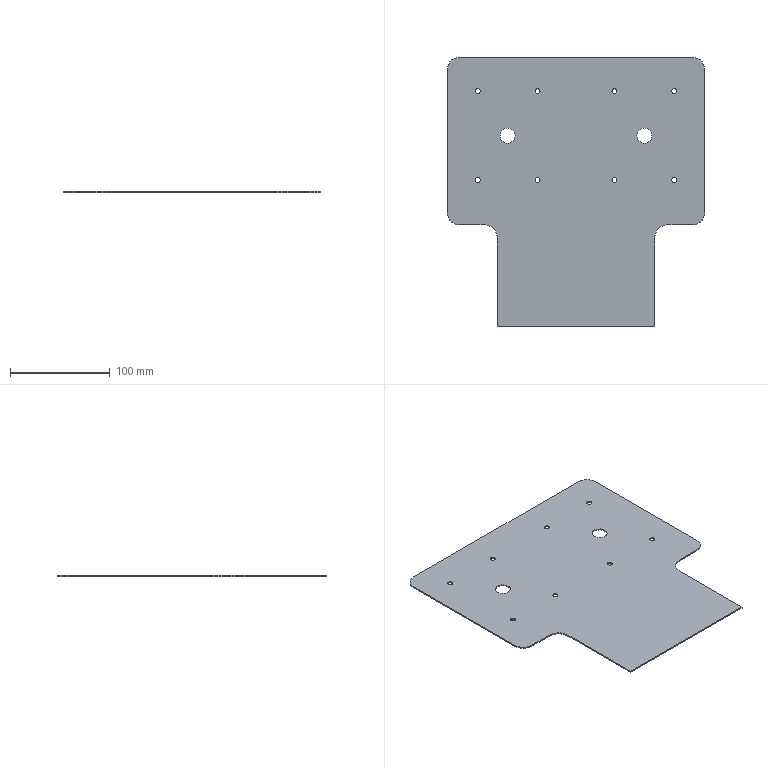Part | SolidWorks | features HoleWzd 2, FlatPattern 1, SMBaseFlange 1, SheetMetal 1 | 1 solid | 36 faces | box 257.6 x 269.6 x 1.2 mm | volume 70428 mm3 | cylinder 26 | plane 10 | commonest cylinder face diameters 5 x16 15 x4 24 x4 26.4 x2
STEP:
#1=CARTESIAN_POINT('',(-33.848,32.78,1.2));
#2=VERTEX_POINT('',#1);
#3=CARTESIAN_POINT('',(-48.848,32.78,1.2));
#4=VERTEX_POINT('',#3);
#5=CARTESIAN_POINT('',(-41.348,32.78,1.2));
#6=DIRECTION('',(0.,0.,-1.));
#7=DIRECTION('',(-1.,0.,0.));
#8=AXIS2_PLACEMENT_3D('',#5,#6,#7);
#9=CIRCLE('',#8,7.5);
#10=EDGE_CURVE('',#2,#4,#9,.T.);
#11=ORIENTED_EDGE('',*,*,#10,.F.);
#12=CARTESIAN_POINT('',(-33.848,32.78,0.));
#13=VERTEX_POINT('',#12);
#14=CARTESIAN_POINT('',(-33.848,32.78,0.));
#15=DIRECTION('',(0.,0.,-1.));
#16=VECTOR('',#15,1000.);
#17=LINE('',#14,#16);
#18=EDGE_CURVE('',#2,#13,#17,.T.);
#19=ORIENTED_EDGE('',*,*,#18,.T.);
#20=CARTESIAN_POINT('',(-48.848,32.78,0.));
#21=VERTEX_POINT('',#20);
#22=CARTESIAN_POINT('',(-41.348,32.78,0.));
#23=DIRECTION('',(0.,0.,-1.));
#24=DIRECTION('',(-1.,0.,0.));
#25=AXIS2_PLACEMENT_3D('',#22,#23,#24);
#26=CIRCLE('',#25,7.5);
#27=EDGE_CURVE('',#13,#21,#26,.T.);
#28=ORIENTED_EDGE('',*,*,#27,.T.);
#29=CARTESIAN_POINT('',(-48.848,32.78,0.));
#30=DIRECTION('',(0.,0.,-1.));
#31=VECTOR('',#30,1000.);
#32=LINE('',#29,#31);
#33=EDGE_CURVE('',#4,#21,#32,.T.);
#34=ORIENTED_EDGE('',*,*,#33,.F.);
#35=EDGE_LOOP('',(#11,#19,#28,#34));
#36=FACE_OUTER_BOUND('',#35,.T.);
#37=CARTESIAN_POINT('',(-41.348,32.78,0.));
#38=DIRECTION('',(0.,0.,-1.));
#39=DIRECTION('',(-1.,0.,0.));
#40=AXIS2_PLACEMENT_3D('',#37,#38,#39);
#41=CYLINDRICAL_SURFACE('',#40,7.5);
#42=ADVANCED_FACE('',(#36),#41,.F.);
#43=CARTESIAN_POINT('',(-170.848,32.78,1.2));
#44=VERTEX_POINT('',#43);
#45=CARTESIAN_POINT('',(-185.848,32.78,1.2));
#46=VERTEX_POINT('',#45);
#47=CARTESIAN_POINT('',(-178.348,32.78,1.2));
#48=DIRECTION('',(0.,0.,-1.));
#49=DIRECTION('',(-1.,0.,0.));
#50=AXIS2_PLACEMENT_3D('',#47,#48,#49);
#51=CIRCLE('',#50,7.5);
#52=EDGE_CURVE('',#44,#46,#51,.T.);
#53=ORIENTED_EDGE('',*,*,#52,.F.);
#54=CARTESIAN_POINT('',(-170.848,32.78,0.));
#55=VERTEX_POINT('',#54);
#56=CARTESIAN_POINT('',(-170.848,32.78,0.));
#57=DIRECTION('',(0.,0.,-1.));
#58=VECTOR('',#57,1000.);
#59=LINE('',#56,#58);
#60=EDGE_CURVE('',#44,#55,#59,.T.);
#61=ORIENTED_EDGE('',*,*,#60,.T.);
#62=CARTESIAN_POINT('',(-185.848,32.78,0.));
#63=VERTEX_POINT('',#62);
#64=CARTESIAN_POINT('',(-178.348,32.78,0.));
#65=DIRECTION('',(0.,0.,-1.));
#66=DIRECTION('',(-1.,0.,0.));
#67=AXIS2_PLACEMENT_3D('',#64,#65,#66);
#68=CIRCLE('',#67,7.5);
#69=EDGE_CURVE('',#55,#63,#68,.T.);
#70=ORIENTED_EDGE('',*,*,#69,.T.);
#71=CARTESIAN_POINT('',(-185.848,32.78,0.));
#72=DIRECTION('',(0.,0.,-1.));
#73=VECTOR('',#72,1000.);
#74=LINE('',#71,#73);
#75=EDGE_CURVE('',#46,#63,#74,.T.);
#76=ORIENTED_EDGE('',*,*,#75,.F.);
#77=EDGE_LOOP('',(#53,#61,#70,#76));
#78=FACE_OUTER_BOUND('',#77,.T.);
#79=CARTESIAN_POINT('',(-178.348,32.78,0.));
#80=DIRECTION('',(0.,0.,-1.));
#81=DIRECTION('',(-1.,0.,0.));
#82=AXIS2_PLACEMENT_3D('',#79,#80,#81);
#83=CYLINDRICAL_SURFACE('',#82,7.5);
#84=ADVANCED_FACE('',(#78),#83,.F.);
#85=CARTESIAN_POINT('',(-8.848,77.28,1.2));
#86=VERTEX_POINT('',#85);
#87=CARTESIAN_POINT('',(-13.848,77.28,1.2));
#88=VERTEX_POINT('',#87);
#89=CARTESIAN_POINT('',(-11.348,77.28,1.2));
#90=DIRECTION('',(0.,0.,-1.));
#91=DIRECTION('',(-1.,0.,0.));
#92=AXIS2_PLACEMENT_3D('',#89,#90,#91);
#93=CIRCLE('',#92,2.5);
#94=EDGE_CURVE('',#86,#88,#93,.T.);
#95=ORIENTED_EDGE('',*,*,#94,.F.);
#96=CARTESIAN_POINT('',(-8.848,77.28,0.));
#97=VERTEX_POINT('',#96);
#98=CARTESIAN_POINT('',(-8.848,77.28,0.));
#99=DIRECTION('',(0.,0.,-1.));
#100=VECTOR('',#99,1000.);
#101=LINE('',#98,#100);
#102=EDGE_CURVE('',#86,#97,#101,.T.);
#103=ORIENTED_EDGE('',*,*,#102,.T.);
#104=CARTESIAN_POINT('',(-13.848,77.28,0.));
#105=VERTEX_POINT('',#104);
#106=CARTESIAN_POINT('',(-11.348,77.28,0.));
#107=DIRECTION('',(0.,0.,-1.));
#108=DIRECTION('',(-1.,0.,0.));
#109=AXIS2_PLACEMENT_3D('',#106,#107,#108);
#110=CIRCLE('',#109,2.5);
#111=EDGE_CURVE('',#97,#105,#110,.T.);
#112=ORIENTED_EDGE('',*,*,#111,.T.);
#113=CARTESIAN_POINT('',(-13.848,77.28,0.));
#114=DIRECTION('',(0.,0.,-1.));
#115=VECTOR('',#114,1000.);
#116=LINE('',#113,#115);
#117=EDGE_CURVE('',#88,#105,#116,.T.);
#118=ORIENTED_EDGE('',*,*,#117,.F.);
#119=EDGE_LOOP('',(#95,#103,#112,#118));
#120=FACE_OUTER_BOUND('',#119,.T.);
#121=CARTESIAN_POINT('',(-11.348,77.28,0.));
#122=DIRECTION('',(0.,0.,-1.));
#123=DIRECTION('',(-1.,0.,0.));
#124=AXIS2_PLACEMENT_3D('',#121,#122,#123);
#125=CYLINDRICAL_SURFACE('',#124,2.5);
#126=ADVANCED_FACE('',(#120),#125,.F.);
#127=CARTESIAN_POINT('',(-8.848,-11.72,1.2));
#128=VERTEX_POINT('',#127);
#129=CARTESIAN_POINT('',(-13.848,-11.72,1.2));
#130=VERTEX_POINT('',#129);
#131=CARTESIAN_POINT('',(-11.348,-11.72,1.2));
#132=DIRECTION('',(0.,0.,-1.));
#133=DIRECTION('',(-1.,0.,0.));
#134=AXIS2_PLACEMENT_3D('',#131,#132,#133);
#135=CIRCLE('',#134,2.5);
#136=EDGE_CURVE('',#128,#130,#135,.T.);
#137=ORIENTED_EDGE('',*,*,#136,.F.);
#138=CARTESIAN_POINT('',(-8.848,-11.72,0.));
#139=VERTEX_POINT('',#138);
#140=CARTESIAN_POINT('',(-8.848,-11.72,0.));
#141=DIRECTION('',(0.,0.,-1.));
#142=VECTOR('',#141,1000.);
#143=LINE('',#140,#142);
#144=EDGE_CURVE('',#128,#139,#143,.T.);
#145=ORIENTED_EDGE('',*,*,#144,.T.);
#146=CARTESIAN_POINT('',(-13.848,-11.72,0.));
#147=VERTEX_POINT('',#146);
#148=CARTESIAN_POINT('',(-11.348,-11.72,0.));
#149=DIRECTION('',(0.,0.,-1.));
#150=DIRECTION('',(-1.,0.,0.));
#151=AXIS2_PLACEMENT_3D('',#148,#149,#150);
#152=CIRCLE('',#151,2.5);
#153=EDGE_CURVE('',#139,#147,#152,.T.);
#154=ORIENTED_EDGE('',*,*,#153,.T.);
#155=CARTESIAN_POINT('',(-13.848,-11.72,0.));
#156=DIRECTION('',(0.,0.,-1.));
#157=VECTOR('',#156,1000.);
#158=LINE('',#155,#157);
#159=EDGE_CURVE('',#130,#147,#158,.T.);
#160=ORIENTED_EDGE('',*,*,#159,.F.);
#161=EDGE_LOOP('',(#137,#145,#154,#160));
#162=FACE_OUTER_BOUND('',#161,.T.);
#163=CARTESIAN_POINT('',(-11.348,-11.72,0.));
#164=DIRECTION('',(0.,0.,-1.));
#165=DIRECTION('',(-1.,0.,0.));
#166=AXIS2_PLACEMENT_3D('',#163,#164,#165);
#167=CYLINDRICAL_SURFACE('',#166,2.5);
#168=ADVANCED_FACE('',(#162),#167,.F.);
#169=CARTESIAN_POINT('',(-68.848,-11.72,1.2));
#170=VERTEX_POINT('',#169);
#171=CARTESIAN_POINT('',(-73.848,-11.72,1.2));
#172=VERTEX_POINT('',#171);
#173=CARTESIAN_POINT('',(-71.348,-11.72,1.2));
#174=DIRECTION('',(0.,0.,-1.));
#175=DIRECTION('',(-1.,0.,0.));
#176=AXIS2_PLACEMENT_3D('',#173,#174,#175);
#177=CIRCLE('',#176,2.5);
#178=EDGE_CURVE('',#170,#172,#177,.T.);
#179=ORIENTED_EDGE('',*,*,#178,.F.);
#180=CARTESIAN_POINT('',(-68.848,-11.72,0.));
#181=VERTEX_POINT('',#180);
#182=CARTESIAN_POINT('',(-68.848,-11.72,0.));
#183=DIRECTION('',(0.,0.,-1.));
#184=VECTOR('',#183,1000.);
#185=LINE('',#182,#184);
#186=EDGE_CURVE('',#170,#181,#185,.T.);
#187=ORIENTED_EDGE('',*,*,#186,.T.);
#188=CARTESIAN_POINT('',(-73.848,-11.72,0.));
#189=VERTEX_POINT('',#188);
#190=CARTESIAN_POINT('',(-71.348,-11.72,0.));
#191=DIRECTION('',(0.,0.,-1.));
#192=DIRECTION('',(-1.,0.,0.));
#193=AXIS2_PLACEMENT_3D('',#190,#191,#192);
#194=CIRCLE('',#193,2.5);
#195=EDGE_CURVE('',#181,#189,#194,.T.);
#196=ORIENTED_EDGE('',*,*,#195,.T.);
#197=CARTESIAN_POINT('',(-73.848,-11.72,0.));
#198=DIRECTION('',(0.,0.,-1.));
#199=VECTOR('',#198,1000.);
#200=LINE('',#197,#199);
#201=EDGE_CURVE('',#172,#189,#200,.T.);
#202=ORIENTED_EDGE('',*,*,#201,.F.);
#203=EDGE_LOOP('',(#179,#187,#196,#202));
#204=FACE_OUTER_BOUND('',#203,.T.);
#205=CARTESIAN_POINT('',(-71.348,-11.72,0.));
#206=DIRECTION('',(0.,0.,-1.));
#207=DIRECTION('',(-1.,0.,0.));
#208=AXIS2_PLACEMENT_3D('',#205,#206,#207);
#209=CYLINDRICAL_SURFACE('',#208,2.5);
#210=ADVANCED_FACE('',(#204),#209,.F.);
#211=CARTESIAN_POINT('',(-68.848,77.28,1.2));
#212=VERTEX_POINT('',#211);
#213=CARTESIAN_POINT('',(-73.848,77.28,1.2));
#214=VERTEX_POINT('',#213);
#215=CARTESIAN_POINT('',(-71.348,77.28,1.2));
#216=DIRECTION('',(0.,0.,-1.));
#217=DIRECTION('',(-1.,0.,0.));
#218=AXIS2_PLACEMENT_3D('',#215,#216,#217);
#219=CIRCLE('',#218,2.5);
#220=EDGE_CURVE('',#212,#214,#219,.T.);
#221=ORIENTED_EDGE('',*,*,#220,.F.);
#222=CARTESIAN_POINT('',(-68.848,77.28,0.));
#223=VERTEX_POINT('',#222);
#224=CARTESIAN_POINT('',(-68.848,77.28,0.));
#225=DIRECTION('',(0.,0.,-1.));
#226=VECTOR('',#225,1000.);
#227=LINE('',#224,#226);
#228=EDGE_CURVE('',#212,#223,#227,.T.);
#229=ORIENTED_EDGE('',*,*,#228,.T.);
#230=CARTESIAN_POINT('',(-73.848,77.28,0.));
#231=VERTEX_POINT('',#230);
#232=CARTESIAN_POINT('',(-71.348,77.28,0.));
#233=DIRECTION('',(0.,0.,-1.));
#234=DIRECTION('',(-1.,0.,0.));
#235=AXIS2_PLACEMENT_3D('',#232,#233,#234);
#236=CIRCLE('',#235,2.5);
#237=EDGE_CURVE('',#223,#231,#236,.T.);
#238=ORIENTED_EDGE('',*,*,#237,.T.);
#239=CARTESIAN_POINT('',(-73.848,77.28,0.));
#240=DIRECTION('',(0.,0.,-1.));
#241=VECTOR('',#240,1000.);
#242=LINE('',#239,#241);
#243=EDGE_CURVE('',#214,#231,#242,.T.);
#244=ORIENTED_EDGE('',*,*,#243,.F.);
#245=EDGE_LOOP('',(#221,#229,#238,#244));
#246=FACE_OUTER_BOUND('',#245,.T.);
#247=CARTESIAN_POINT('',(-71.348,77.28,0.));
#248=DIRECTION('',(0.,0.,-1.));
#249=DIRECTION('',(-1.,0.,0.));
#250=AXIS2_PLACEMENT_3D('',#247,#248,#249);
#251=CYLINDRICAL_SURFACE('',#250,2.5);
#252=ADVANCED_FACE('',(#246),#251,.F.);
#253=CARTESIAN_POINT('',(-145.848,77.28,1.2));
#254=VERTEX_POINT('',#253);
#255=CARTESIAN_POINT('',(-150.848,77.28,1.2));
#256=VERTEX_POINT('',#255);
#257=CARTESIAN_POINT('',(-148.348,77.28,1.2));
#258=DIRECTION('',(0.,0.,-1.));
#259=DIRECTION('',(-1.,0.,0.));
#260=AXIS2_PLACEMENT_3D('',#257,#258,#259);
#261=CIRCLE('',#260,2.5);
#262=EDGE_CURVE('',#254,#256,#261,.T.);
#263=ORIENTED_EDGE('',*,*,#262,.F.);
#264=CARTESIAN_POINT('',(-145.848,77.28,0.));
#265=VERTEX_POINT('',#264);
#266=CARTESIAN_POINT('',(-145.848,77.28,0.));
#267=DIRECTION('',(0.,0.,-1.));
#268=VECTOR('',#267,1000.);
#269=LINE('',#266,#268);
#270=EDGE_CURVE('',#254,#265,#269,.T.);
#271=ORIENTED_EDGE('',*,*,#270,.T.);
#272=CARTESIAN_POINT('',(-150.848,77.28,0.));
#273=VERTEX_POINT('',#272);
#274=CARTESIAN_POINT('',(-148.348,77.28,0.));
#275=DIRECTION('',(0.,0.,-1.));
#276=DIRECTION('',(-1.,0.,0.));
#277=AXIS2_PLACEMENT_3D('',#274,#275,#276);
#278=CIRCLE('',#277,2.5);
#279=EDGE_CURVE('',#265,#273,#278,.T.);
#280=ORIENTED_EDGE('',*,*,#279,.T.);
#281=CARTESIAN_POINT('',(-150.848,77.28,0.));
#282=DIRECTION('',(0.,0.,-1.));
#283=VECTOR('',#282,1000.);
#284=LINE('',#281,#283);
#285=EDGE_CURVE('',#256,#273,#284,.T.);
#286=ORIENTED_EDGE('',*,*,#285,.F.);
#287=EDGE_LOOP('',(#263,#271,#280,#286));
#288=FACE_OUTER_BOUND('',#287,.T.);
#289=CARTESIAN_POINT('',(-148.348,77.28,0.));
#290=DIRECTION('',(0.,0.,-1.));
#291=DIRECTION('',(-1.,0.,0.));
#292=AXIS2_PLACEMENT_3D('',#289,#290,#291);
#293=CYLINDRICAL_SURFACE('',#292,2.5);
#294=ADVANCED_FACE('',(#288),#293,.F.);
#295=CARTESIAN_POINT('',(-145.848,-11.72,1.2));
#296=VERTEX_POINT('',#295);
#297=CARTESIAN_POINT('',(-150.848,-11.72,1.2));
#298=VERTEX_POINT('',#297);
#299=CARTESIAN_POINT('',(-148.348,-11.72,1.2));
#300=DIRECTION('',(0.,0.,-1.));
#301=DIRECTION('',(-1.,0.,0.));
#302=AXIS2_PLACEMENT_3D('',#299,#300,#301);
#303=CIRCLE('',#302,2.5);
#304=EDGE_CURVE('',#296,#298,#303,.T.);
#305=ORIENTED_EDGE('',*,*,#304,.F.);
#306=CARTESIAN_POINT('',(-145.848,-11.72,0.));
#307=VERTEX_POINT('',#306);
#308=CARTESIAN_POINT('',(-145.848,-11.72,0.));
#309=DIRECTION('',(0.,0.,-1.));
#310=VECTOR('',#309,1000.);
#311=LINE('',#308,#310);
#312=EDGE_CURVE('',#296,#307,#311,.T.);
#313=ORIENTED_EDGE('',*,*,#312,.T.);
#314=CARTESIAN_POINT('',(-150.848,-11.72,0.));
#315=VERTEX_POINT('',#314);
#316=CARTESIAN_POINT('',(-148.348,-11.72,0.));
#317=DIRECTION('',(0.,0.,-1.));
#318=DIRECTION('',(-1.,0.,0.));
#319=AXIS2_PLACEMENT_3D('',#316,#317,#318);
#320=CIRCLE('',#319,2.5);
#321=EDGE_CURVE('',#307,#315,#320,.T.);
#322=ORIENTED_EDGE('',*,*,#321,.T.);
#323=CARTESIAN_POINT('',(-150.848,-11.72,0.));
#324=DIRECTION('',(0.,0.,-1.));
#325=VECTOR('',#324,1000.);
#326=LINE('',#323,#325);
#327=EDGE_CURVE('',#298,#315,#326,.T.);
#328=ORIENTED_EDGE('',*,*,#327,.F.);
#329=EDGE_LOOP('',(#305,#313,#322,#328));
#330=FACE_OUTER_BOUND('',#329,.T.);
#331=CARTESIAN_POINT('',(-148.348,-11.72,0.));
#332=DIRECTION('',(0.,0.,-1.));
#333=DIRECTION('',(-1.,0.,0.));
#334=AXIS2_PLACEMENT_3D('',#331,#332,#333);
#335=CYLINDRICAL_SURFACE('',#334,2.5);
#336=ADVANCED_FACE('',(#330),#335,.F.);
#337=CARTESIAN_POINT('',(-205.848,-11.72,1.2));
#338=VERTEX_POINT('',#337);
#339=CARTESIAN_POINT('',(-210.848,-11.72,1.2));
#340=VERTEX_POINT('',#339);
#341=CARTESIAN_POINT('',(-208.348,-11.72,1.2));
#342=DIRECTION('',(0.,0.,-1.));
#343=DIRECTION('',(-1.,0.,0.));
#344=AXIS2_PLACEMENT_3D('',#341,#342,#343);
#345=CIRCLE('',#344,2.5);
#346=EDGE_CURVE('',#338,#340,#345,.T.);
#347=ORIENTED_EDGE('',*,*,#346,.F.);
#348=CARTESIAN_POINT('',(-205.848,-11.72,0.));
#349=VERTEX_POINT('',#348);
#350=CARTESIAN_POINT('',(-205.848,-11.72,0.));
#351=DIRECTION('',(0.,0.,-1.));
#352=VECTOR('',#351,1000.);
#353=LINE('',#350,#352);
#354=EDGE_CURVE('',#338,#349,#353,.T.);
#355=ORIENTED_EDGE('',*,*,#354,.T.);
#356=CARTESIAN_POINT('',(-210.848,-11.72,0.));
#357=VERTEX_POINT('',#356);
#358=CARTESIAN_POINT('',(-208.348,-11.72,0.));
#359=DIRECTION('',(0.,0.,-1.));
#360=DIRECTION('',(-1.,0.,0.));
#361=AXIS2_PLACEMENT_3D('',#358,#359,#360);
#362=CIRCLE('',#361,2.5);
#363=EDGE_CURVE('',#349,#357,#362,.T.);
#364=ORIENTED_EDGE('',*,*,#363,.T.);
#365=CARTESIAN_POINT('',(-210.848,-11.72,0.));
#366=DIRECTION('',(0.,0.,-1.));
#367=VECTOR('',#366,1000.);
#368=LINE('',#365,#367);
#369=EDGE_CURVE('',#340,#357,#368,.T.);
#370=ORIENTED_EDGE('',*,*,#369,.F.);
#371=EDGE_LOOP('',(#347,#355,#364,#370));
#372=FACE_OUTER_BOUND('',#371,.T.);
#373=CARTESIAN_POINT('',(-208.348,-11.72,0.));
#374=DIRECTION('',(0.,0.,-1.));
#375=DIRECTION('',(-1.,0.,0.));
#376=AXIS2_PLACEMENT_3D('',#373,#374,#375);
#377=CYLINDRICAL_SURFACE('',#376,2.5);
#378=ADVANCED_FACE('',(#372),#377,.F.);
#379=CARTESIAN_POINT('',(-205.848,77.28,1.2));
#380=VERTEX_POINT('',#379);
#381=CARTESIAN_POINT('',(-210.848,77.28,1.2));
#382=VERTEX_POINT('',#381);
#383=CARTESIAN_POINT('',(-208.348,77.28,1.2));
#384=DIRECTION('',(0.,0.,-1.));
#385=DIRECTION('',(-1.,0.,0.));
#386=AXIS2_PLACEMENT_3D('',#383,#384,#385);
#387=CIRCLE('',#386,2.5);
#388=EDGE_CURVE('',#380,#382,#387,.T.);
#389=ORIENTED_EDGE('',*,*,#388,.F.);
#390=CARTESIAN_POINT('',(-205.848,77.28,0.));
#391=VERTEX_POINT('',#390);
#392=CARTESIAN_POINT('',(-205.848,77.28,0.));
#393=DIRECTION('',(0.,0.,-1.));
#394=VECTOR('',#393,1000.);
#395=LINE('',#392,#394);
#396=EDGE_CURVE('',#380,#391,#395,.T.);
#397=ORIENTED_EDGE('',*,*,#396,.T.);
#398=CARTESIAN_POINT('',(-210.848,77.28,0.));
#399=VERTEX_POINT('',#398);
#400=CARTESIAN_POINT('',(-208.348,77.28,0.));
#401=DIRECTION('',(0.,0.,-1.));
#402=DIRECTION('',(-1.,0.,0.));
#403=AXIS2_PLACEMENT_3D('',#400,#401,#402);
#404=CIRCLE('',#403,2.5);
#405=EDGE_CURVE('',#391,#399,#404,.T.);
#406=ORIENTED_EDGE('',*,*,#405,.T.);
#407=CARTESIAN_POINT('',(-210.848,77.28,0.));
#408=DIRECTION('',(0.,0.,-1.));
#409=VECTOR('',#408,1000.);
#410=LINE('',#407,#409);
#411=EDGE_CURVE('',#382,#399,#410,.T.);
#412=ORIENTED_EDGE('',*,*,#411,.F.);
#413=EDGE_LOOP('',(#389,#397,#406,#412));
#414=FACE_OUTER_BOUND('',#413,.T.);
#415=CARTESIAN_POINT('',(-208.348,77.28,0.));
#416=DIRECTION('',(0.,0.,-1.));
#417=DIRECTION('',(-1.,0.,0.));
#418=AXIS2_PLACEMENT_3D('',#415,#416,#417);
#419=CYLINDRICAL_SURFACE('',#418,2.5);
#420=ADVANCED_FACE('',(#414),#419,.F.);
#421=CARTESIAN_POINT('',(6.952,111.08,0.));
#422=VERTEX_POINT('',#421);
#423=CARTESIAN_POINT('',(18.952,99.08,0.));
#424=VERTEX_POINT('',#423);
#425=CARTESIAN_POINT('',(6.952,99.08,0.));
#426=DIRECTION('',(0.,0.,-1.));
#427=DIRECTION('',(-1.,0.,0.));
#428=AXIS2_PLACEMENT_3D('',#425,#426,#427);
#429=CIRCLE('',#428,12.);
#430=EDGE_CURVE('',#422,#424,#429,.T.);
#431=ORIENTED_EDGE('',*,*,#430,.F.);
#432=CARTESIAN_POINT('',(6.952,111.08,1.2));
#433=VERTEX_POINT('',#432);
#434=CARTESIAN_POINT('',(6.952,111.08,1.2));
#435=DIRECTION('',(0.,0.,-1.));
#436=VECTOR('',#435,1000.);
#437=LINE('',#434,#436);
#438=EDGE_CURVE('',#433,#422,#437,.T.);
#439=ORIENTED_EDGE('',*,*,#438,.F.);
#440=CARTESIAN_POINT('',(18.952,99.08,1.2));
#441=VERTEX_POINT('',#440);
#442=CARTESIAN_POINT('',(6.952,99.08,1.2));
#443=DIRECTION('',(0.,0.,-1.));
#444=DIRECTION('',(-1.,0.,0.));
#445=AXIS2_PLACEMENT_3D('',#442,#443,#444);
#446=CIRCLE('',#445,12.);
#447=EDGE_CURVE('',#433,#441,#446,.T.);
#448=ORIENTED_EDGE('',*,*,#447,.T.);
#449=CARTESIAN_POINT('',(18.952,99.08,1.2));
#450=DIRECTION('',(0.,0.,-1.));
#451=VECTOR('',#450,1000.);
#452=LINE('',#449,#451);
#453=EDGE_CURVE('',#441,#424,#452,.T.);
#454=ORIENTED_EDGE('',*,*,#453,.T.);
#455=EDGE_LOOP('',(#431,#439,#448,#454));
#456=FACE_OUTER_BOUND('',#455,.T.);
#457=CARTESIAN_POINT('',(6.952,99.08,1.2));
#458=DIRECTION('',(0.,0.,-1.));
#459=DIRECTION('',(-1.,0.,0.));
#460=AXIS2_PLACEMENT_3D('',#457,#458,#459);
#461=CYLINDRICAL_SURFACE('',#460,12.);
#462=ADVANCED_FACE('',(#456),#461,.T.);
#463=CARTESIAN_POINT('',(-226.648,111.08,0.));
#464=VERTEX_POINT('',#463);
#465=CARTESIAN_POINT('',(-226.648,111.08,0.));
#466=DIRECTION('',(1.,0.,0.));
#467=VECTOR('',#466,1000.);
#468=LINE('',#465,#467);
#469=EDGE_CURVE('',#464,#422,#468,.T.);
#470=ORIENTED_EDGE('',*,*,#469,.F.);
#471=CARTESIAN_POINT('',(-226.648,111.08,1.2));
#472=VERTEX_POINT('',#471);
#473=CARTESIAN_POINT('',(-226.648,111.08,1.2));
#474=DIRECTION('',(0.,0.,-1.));
#475=VECTOR('',#474,1000.);
#476=LINE('',#473,#475);
#477=EDGE_CURVE('',#472,#464,#476,.T.);
#478=ORIENTED_EDGE('',*,*,#477,.F.);
#479=CARTESIAN_POINT('',(-226.648,111.08,1.2));
#480=DIRECTION('',(1.,0.,0.));
#481=VECTOR('',#480,1000.);
#482=LINE('',#479,#481);
#483=EDGE_CURVE('',#472,#433,#482,.T.);
#484=ORIENTED_EDGE('',*,*,#483,.T.);
#485=ORIENTED_EDGE('',*,*,#438,.T.);
#486=EDGE_LOOP('',(#470,#478,#484,#485));
#487=FACE_OUTER_BOUND('',#486,.T.);
#488=CARTESIAN_POINT('',(-226.648,111.08,1.2));
#489=DIRECTION('',(0.,1.,0.));
#490=DIRECTION('',(-1.,0.,0.));
#491=AXIS2_PLACEMENT_3D('',#488,#489,#490);
#492=PLANE('',#491);
#493=ADVANCED_FACE('',(#487),#492,.T.);
#494=CARTESIAN_POINT('',(-238.648,99.08,0.));
#495=VERTEX_POINT('',#494);
#496=CARTESIAN_POINT('',(-226.648,99.08,0.));
#497=DIRECTION('',(0.,0.,-1.));
#498=DIRECTION('',(-1.,0.,0.));
#499=AXIS2_PLACEMENT_3D('',#496,#497,#498);
#500=CIRCLE('',#499,12.);
#501=EDGE_CURVE('',#495,#464,#500,.T.);
#502=ORIENTED_EDGE('',*,*,#501,.F.);
#503=CARTESIAN_POINT('',(-238.648,99.08,1.2));
#504=VERTEX_POINT('',#503);
#505=CARTESIAN_POINT('',(-238.648,99.08,1.2));
#506=DIRECTION('',(0.,0.,-1.));
#507=VECTOR('',#506,1000.);
#508=LINE('',#505,#507);
#509=EDGE_CURVE('',#504,#495,#508,.T.);
#510=ORIENTED_EDGE('',*,*,#509,.F.);
#511=CARTESIAN_POINT('',(-226.648,99.08,1.2));
#512=DIRECTION('',(0.,0.,-1.));
#513=DIRECTION('',(-1.,0.,0.));
#514=AXIS2_PLACEMENT_3D('',#511,#512,#513);
#515=CIRCLE('',#514,12.);
#516=EDGE_CURVE('',#504,#472,#515,.T.);
#517=ORIENTED_EDGE('',*,*,#516,.T.);
#518=ORIENTED_EDGE('',*,*,#477,.T.);
#519=EDGE_LOOP('',(#502,#510,#517,#518));
#520=FACE_OUTER_BOUND('',#519,.T.);
#521=CARTESIAN_POINT('',(-226.648,99.08,1.2));
#522=DIRECTION('',(0.,0.,-1.));
#523=DIRECTION('',(-1.,0.,0.));
#524=AXIS2_PLACEMENT_3D('',#521,#522,#523);
#525=CYLINDRICAL_SURFACE('',#524,12.);
#526=ADVANCED_FACE('',(#520),#525,.T.);
#527=CARTESIAN_POINT('',(-238.648,-44.52,0.));
#528=VERTEX_POINT('',#527);
#529=CARTESIAN_POINT('',(-238.648,-44.52,0.));
#530=DIRECTION('',(0.,1.,0.));
#531=VECTOR('',#530,1000.);
#532=LINE('',#529,#531);
#533=EDGE_CURVE('',#528,#495,#532,.T.);
#534=ORIENTED_EDGE('',*,*,#533,.F.);
#535=CARTESIAN_POINT('',(-238.648,-44.52,1.2));
#536=VERTEX_POINT('',#535);
#537=CARTESIAN_POINT('',(-238.648,-44.52,1.2));
#538=DIRECTION('',(0.,0.,-1.));
#539=VECTOR('',#538,1000.);
#540=LINE('',#537,#539);
#541=EDGE_CURVE('',#536,#528,#540,.T.);
#542=ORIENTED_EDGE('',*,*,#541,.F.);
#543=CARTESIAN_POINT('',(-238.648,-44.52,1.2));
#544=DIRECTION('',(0.,1.,0.));
#545=VECTOR('',#544,1000.);
#546=LINE('',#543,#545);
#547=EDGE_CURVE('',#536,#504,#546,.T.);
#548=ORIENTED_EDGE('',*,*,#547,.T.);
#549=ORIENTED_EDGE('',*,*,#509,.T.);
#550=EDGE_LOOP('',(#534,#542,#548,#549));
#551=FACE_OUTER_BOUND('',#550,.T.);
#552=CARTESIAN_POINT('',(-238.648,-44.52,1.2));
#553=DIRECTION('',(-1.,0.,0.));
#554=DIRECTION('',(0.,-1.,0.));
#555=AXIS2_PLACEMENT_3D('',#552,#553,#554);
#556=PLANE('',#555);
#557=ADVANCED_FACE('',(#551),#556,.T.);
#558=CARTESIAN_POINT('',(-226.648,-56.52,0.));
#559=VERTEX_POINT('',#558);
#560=CARTESIAN_POINT('',(-226.648,-44.52,0.));
#561=DIRECTION('',(0.,0.,-1.));
#562=DIRECTION('',(-1.,0.,0.));
#563=AXIS2_PLACEMENT_3D('',#560,#561,#562);
#564=CIRCLE('',#563,12.);
#565=EDGE_CURVE('',#559,#528,#564,.T.);
#566=ORIENTED_EDGE('',*,*,#565,.F.);
#567=CARTESIAN_POINT('',(-226.648,-56.52,1.2));
#568=VERTEX_POINT('',#567);
#569=CARTESIAN_POINT('',(-226.648,-56.52,1.2));
#570=DIRECTION('',(0.,0.,-1.));
#571=VECTOR('',#570,1000.);
#572=LINE('',#569,#571);
#573=EDGE_CURVE('',#568,#559,#572,.T.);
#574=ORIENTED_EDGE('',*,*,#573,.F.);
#575=CARTESIAN_POINT('',(-226.648,-44.52,1.2));
#576=DIRECTION('',(0.,0.,-1.));
#577=DIRECTION('',(-1.,0.,0.));
#578=AXIS2_PLACEMENT_3D('',#575,#576,#577);
#579=CIRCLE('',#578,12.);
#580=EDGE_CURVE('',#568,#536,#579,.T.);
#581=ORIENTED_EDGE('',*,*,#580,.T.);
#582=ORIENTED_EDGE('',*,*,#541,.T.);
#583=EDGE_LOOP('',(#566,#574,#581,#582));
#584=FACE_OUTER_BOUND('',#583,.T.);
#585=CARTESIAN_POINT('',(-226.648,-44.52,1.2));
#586=DIRECTION('',(0.,0.,-1.));
#587=DIRECTION('',(-1.,0.,0.));
#588=AXIS2_PLACEMENT_3D('',#585,#586,#587);
#589=CYLINDRICAL_SURFACE('',#588,12.);
#590=ADVANCED_FACE('',(#584),#589,.T.);
#591=CARTESIAN_POINT('',(-201.848,-56.52,0.));
#592=VERTEX_POINT('',#591);
#593=CARTESIAN_POINT('',(-201.848,-56.52,0.));
#594=DIRECTION('',(-1.,0.,0.));
#595=VECTOR('',#594,1000.);
#596=LINE('',#593,#595);
#597=EDGE_CURVE('',#592,#559,#596,.T.);
#598=ORIENTED_EDGE('',*,*,#597,.F.);
#599=CARTESIAN_POINT('',(-201.848,-56.52,1.2));
#600=VERTEX_POINT('',#599);
#601=CARTESIAN_POINT('',(-201.848,-56.52,1.2));
#602=DIRECTION('',(0.,0.,-1.));
#603=VECTOR('',#602,1000.);
#604=LINE('',#601,#603);
#605=EDGE_CURVE('',#600,#592,#604,.T.);
#606=ORIENTED_EDGE('',*,*,#605,.F.);
#607=CARTESIAN_POINT('',(-201.848,-56.52,1.2));
#608=DIRECTION('',(-1.,0.,0.));
#609=VECTOR('',#608,1000.);
#610=LINE('',#607,#609);
#611=EDGE_CURVE('',#600,#568,#610,.T.);
#612=ORIENTED_EDGE('',*,*,#611,.T.);
#613=ORIENTED_EDGE('',*,*,#573,.T.);
#614=EDGE_LOOP('',(#598,#606,#612,#613));
#615=FACE_OUTER_BOUND('',#614,.T.);
#616=CARTESIAN_POINT('',(-201.848,-56.52,1.2));
#617=DIRECTION('',(0.,-1.,0.));
#618=DIRECTION('',(0.,0.,-1.));
#619=AXIS2_PLACEMENT_3D('',#616,#617,#618);
#620=PLANE('',#619);
#621=ADVANCED_FACE('',(#615),#620,.T.);
#622=CARTESIAN_POINT('',(-188.648,-69.72,0.));
#623=VERTEX_POINT('',#622);
#624=CARTESIAN_POINT('',(-201.848,-69.72,0.));
#625=DIRECTION('',(0.,0.,1.));
#626=DIRECTION('',(1.,0.,0.));
#627=AXIS2_PLACEMENT_3D('',#624,#625,#626);
#628=CIRCLE('',#627,13.2);
#629=EDGE_CURVE('',#623,#592,#628,.T.);
#630=ORIENTED_EDGE('',*,*,#629,.F.);
#631=CARTESIAN_POINT('',(-188.648,-69.72,1.2));
#632=VERTEX_POINT('',#631);
#633=CARTESIAN_POINT('',(-188.648,-69.72,1.2));
#634=DIRECTION('',(0.,0.,-1.));
#635=VECTOR('',#634,1000.);
#636=LINE('',#633,#635);
#637=EDGE_CURVE('',#632,#623,#636,.T.);
#638=ORIENTED_EDGE('',*,*,#637,.F.);
#639=CARTESIAN_POINT('',(-201.848,-69.72,1.2));
#640=DIRECTION('',(0.,0.,1.));
#641=DIRECTION('',(1.,0.,0.));
#642=AXIS2_PLACEMENT_3D('',#639,#640,#641);
#643=CIRCLE('',#642,13.2);
#644=EDGE_CURVE('',#632,#600,#643,.T.);
#645=ORIENTED_EDGE('',*,*,#644,.T.);
#646=ORIENTED_EDGE('',*,*,#605,.T.);
#647=EDGE_LOOP('',(#630,#638,#645,#646));
#648=FACE_OUTER_BOUND('',#647,.T.);
#649=CARTESIAN_POINT('',(-201.848,-69.72,1.2));
#650=DIRECTION('',(0.,0.,-1.));
#651=DIRECTION('',(-1.,0.,0.));
#652=AXIS2_PLACEMENT_3D('',#649,#650,#651);
#653=CYLINDRICAL_SURFACE('',#652,13.2);
#654=ADVANCED_FACE('',(#648),#653,.F.);
#655=CARTESIAN_POINT('',(-188.648,-158.52,0.));
#656=VERTEX_POINT('',#655);
#657=CARTESIAN_POINT('',(-188.648,-158.52,0.));
#658=DIRECTION('',(0.,1.,0.));
#659=VECTOR('',#658,1000.);
#660=LINE('',#657,#659);
#661=EDGE_CURVE('',#656,#623,#660,.T.);
#662=ORIENTED_EDGE('',*,*,#661,.F.);
#663=CARTESIAN_POINT('',(-188.648,-158.52,1.2));
#664=VERTEX_POINT('',#663);
#665=CARTESIAN_POINT('',(-188.648,-158.52,1.2));
#666=DIRECTION('',(0.,0.,-1.));
#667=VECTOR('',#666,1000.);
#668=LINE('',#665,#667);
#669=EDGE_CURVE('',#664,#656,#668,.T.);
#670=ORIENTED_EDGE('',*,*,#669,.F.);
#671=CARTESIAN_POINT('',(-188.648,-158.52,1.2));
#672=DIRECTION('',(0.,1.,0.));
#673=VECTOR('',#672,1000.);
#674=LINE('',#671,#673);
#675=EDGE_CURVE('',#664,#632,#674,.T.);
#676=ORIENTED_EDGE('',*,*,#675,.T.);
#677=ORIENTED_EDGE('',*,*,#637,.T.);
#678=EDGE_LOOP('',(#662,#670,#676,#677));
#679=FACE_OUTER_BOUND('',#678,.T.);
#680=CARTESIAN_POINT('',(-188.648,-158.52,1.2));
#681=DIRECTION('',(-1.,0.,0.));
#682=DIRECTION('',(0.,0.,1.));
#683=AXIS2_PLACEMENT_3D('',#680,#681,#682);
#684=PLANE('',#683);
#685=ADVANCED_FACE('',(#679),#684,.T.);
#686=CARTESIAN_POINT('',(-31.048,-158.52,0.));
#687=VERTEX_POINT('',#686);
#688=CARTESIAN_POINT('',(-31.048,-158.52,0.));
#689=DIRECTION('',(-1.,0.,0.));
#690=VECTOR('',#689,1000.);
#691=LINE('',#688,#690);
#692=EDGE_CURVE('',#687,#656,#691,.T.);
#693=ORIENTED_EDGE('',*,*,#692,.F.);
#694=CARTESIAN_POINT('',(-31.048,-158.52,1.2));
#695=VERTEX_POINT('',#694);
#696=CARTESIAN_POINT('',(-31.048,-158.52,1.2));
#697=DIRECTION('',(0.,0.,-1.));
#698=VECTOR('',#697,1000.);
#699=LINE('',#696,#698);
#700=EDGE_CURVE('',#695,#687,#699,.T.);
#701=ORIENTED_EDGE('',*,*,#700,.F.);
#702=CARTESIAN_POINT('',(-31.048,-158.52,1.2));
#703=DIRECTION('',(-1.,0.,0.));
#704=VECTOR('',#703,1000.);
#705=LINE('',#702,#704);
#706=EDGE_CURVE('',#695,#664,#705,.T.);
#707=ORIENTED_EDGE('',*,*,#706,.T.);
#708=ORIENTED_EDGE('',*,*,#669,.T.);
#709=EDGE_LOOP('',(#693,#701,#707,#708));
#710=FACE_OUTER_BOUND('',#709,.T.);
#711=CARTESIAN_POINT('',(-31.048,-158.52,1.2));
#712=DIRECTION('',(0.,-1.,0.));
#713=DIRECTION('',(0.,0.,-1.));
#714=AXIS2_PLACEMENT_3D('',#711,#712,#713);
#715=PLANE('',#714);
#716=ADVANCED_FACE('',(#710),#715,.T.);
#717=CARTESIAN_POINT('',(-31.048,-69.72,0.));
#718=VERTEX_POINT('',#717);
#719=CARTESIAN_POINT('',(-31.048,-69.72,0.));
#720=DIRECTION('',(0.,-1.,0.));
#721=VECTOR('',#720,1000.);
#722=LINE('',#719,#721);
#723=EDGE_CURVE('',#718,#687,#722,.T.);
#724=ORIENTED_EDGE('',*,*,#723,.F.);
#725=CARTESIAN_POINT('',(-31.048,-69.72,1.2));
#726=VERTEX_POINT('',#725);
#727=CARTESIAN_POINT('',(-31.048,-69.72,1.2));
#728=DIRECTION('',(0.,0.,-1.));
#729=VECTOR('',#728,1000.);
#730=LINE('',#727,#729);
#731=EDGE_CURVE('',#726,#718,#730,.T.);
#732=ORIENTED_EDGE('',*,*,#731,.F.);
#733=CARTESIAN_POINT('',(-31.048,-69.72,1.2));
#734=DIRECTION('',(0.,-1.,0.));
#735=VECTOR('',#734,1000.);
#736=LINE('',#733,#735);
#737=EDGE_CURVE('',#726,#695,#736,.T.);
#738=ORIENTED_EDGE('',*,*,#737,.T.);
#739=ORIENTED_EDGE('',*,*,#700,.T.);
#740=EDGE_LOOP('',(#724,#732,#738,#739));
#741=FACE_OUTER_BOUND('',#740,.T.);
#742=CARTESIAN_POINT('',(-31.048,-69.72,1.2));
#743=DIRECTION('',(1.,0.,0.));
#744=DIRECTION('',(0.,1.,0.));
#745=AXIS2_PLACEMENT_3D('',#742,#743,#744);
#746=PLANE('',#745);
#747=ADVANCED_FACE('',(#741),#746,.T.);
#748=CARTESIAN_POINT('',(-17.848,-56.52,0.));
#749=VERTEX_POINT('',#748);
#750=CARTESIAN_POINT('',(-17.848,-69.72,0.));
#751=DIRECTION('',(0.,0.,1.));
#752=DIRECTION('',(1.,0.,0.));
#753=AXIS2_PLACEMENT_3D('',#750,#751,#752);
#754=CIRCLE('',#753,13.2);
#755=EDGE_CURVE('',#749,#718,#754,.T.);
#756=ORIENTED_EDGE('',*,*,#755,.F.);
#757=CARTESIAN_POINT('',(-17.848,-56.52,1.2));
#758=VERTEX_POINT('',#757);
#759=CARTESIAN_POINT('',(-17.848,-56.52,1.2));
#760=DIRECTION('',(0.,0.,-1.));
#761=VECTOR('',#760,1000.);
#762=LINE('',#759,#761);
#763=EDGE_CURVE('',#758,#749,#762,.T.);
#764=ORIENTED_EDGE('',*,*,#763,.F.);
#765=CARTESIAN_POINT('',(-17.848,-69.72,1.2));
#766=DIRECTION('',(0.,0.,1.));
#767=DIRECTION('',(1.,0.,0.));
#768=AXIS2_PLACEMENT_3D('',#765,#766,#767);
#769=CIRCLE('',#768,13.2);
#770=EDGE_CURVE('',#758,#726,#769,.T.);
#771=ORIENTED_EDGE('',*,*,#770,.T.);
#772=ORIENTED_EDGE('',*,*,#731,.T.);
#773=EDGE_LOOP('',(#756,#764,#771,#772));
#774=FACE_OUTER_BOUND('',#773,.T.);
#775=CARTESIAN_POINT('',(-17.848,-69.72,1.2));
#776=DIRECTION('',(0.,0.,-1.));
#777=DIRECTION('',(-1.,0.,0.));
#778=AXIS2_PLACEMENT_3D('',#775,#776,#777);
#779=CYLINDRICAL_SURFACE('',#778,13.2);
#780=ADVANCED_FACE('',(#774),#779,.F.);
#781=CARTESIAN_POINT('',(6.952,-56.52,0.));
#782=VERTEX_POINT('',#781);
#783=CARTESIAN_POINT('',(6.952,-56.52,0.));
#784=DIRECTION('',(-1.,0.,0.));
#785=VECTOR('',#784,1000.);
#786=LINE('',#783,#785);
#787=EDGE_CURVE('',#782,#749,#786,.T.);
#788=ORIENTED_EDGE('',*,*,#787,.F.);
#789=CARTESIAN_POINT('',(6.952,-56.52,1.2));
#790=VERTEX_POINT('',#789);
#791=CARTESIAN_POINT('',(6.952,-56.52,1.2));
#792=DIRECTION('',(0.,0.,-1.));
#793=VECTOR('',#792,1000.);
#794=LINE('',#791,#793);
#795=EDGE_CURVE('',#790,#782,#794,.T.);
#796=ORIENTED_EDGE('',*,*,#795,.F.);
#797=CARTESIAN_POINT('',(6.952,-56.52,1.2));
#798=DIRECTION('',(-1.,0.,0.));
#799=VECTOR('',#798,1000.);
#800=LINE('',#797,#799);
#801=EDGE_CURVE('',#790,#758,#800,.T.);
#802=ORIENTED_EDGE('',*,*,#801,.T.);
#803=ORIENTED_EDGE('',*,*,#763,.T.);
#804=EDGE_LOOP('',(#788,#796,#802,#803));
#805=FACE_OUTER_BOUND('',#804,.T.);
#806=CARTESIAN_POINT('',(6.952,-56.52,1.2));
#807=DIRECTION('',(0.,-1.,0.));
#808=DIRECTION('',(1.,0.,0.));
#809=AXIS2_PLACEMENT_3D('',#806,#807,#808);
#810=PLANE('',#809);
#811=ADVANCED_FACE('',(#805),#810,.T.);
#812=CARTESIAN_POINT('',(18.952,-44.52,0.));
#813=VERTEX_POINT('',#812);
#814=CARTESIAN_POINT('',(6.952,-44.52,0.));
#815=DIRECTION('',(0.,0.,-1.));
#816=DIRECTION('',(-1.,0.,0.));
#817=AXIS2_PLACEMENT_3D('',#814,#815,#816);
#818=CIRCLE('',#817,12.);
#819=EDGE_CURVE('',#813,#782,#818,.T.);
#820=ORIENTED_EDGE('',*,*,#819,.F.);
#821=CARTESIAN_POINT('',(18.952,-44.52,1.2));
#822=VERTEX_POINT('',#821);
#823=CARTESIAN_POINT('',(18.952,-44.52,1.2));
#824=DIRECTION('',(0.,0.,-1.));
#825=VECTOR('',#824,1000.);
#826=LINE('',#823,#825);
#827=EDGE_CURVE('',#822,#813,#826,.T.);
#828=ORIENTED_EDGE('',*,*,#827,.F.);
#829=CARTESIAN_POINT('',(6.952,-44.52,1.2));
#830=DIRECTION('',(0.,0.,-1.));
#831=DIRECTION('',(-1.,0.,0.));
#832=AXIS2_PLACEMENT_3D('',#829,#830,#831);
#833=CIRCLE('',#832,12.);
#834=EDGE_CURVE('',#822,#790,#833,.T.);
#835=ORIENTED_EDGE('',*,*,#834,.T.);
#836=ORIENTED_EDGE('',*,*,#795,.T.);
#837=EDGE_LOOP('',(#820,#828,#835,#836));
#838=FACE_OUTER_BOUND('',#837,.T.);
#839=CARTESIAN_POINT('',(6.952,-44.52,1.2));
#840=DIRECTION('',(0.,0.,-1.));
#841=DIRECTION('',(-1.,0.,0.));
#842=AXIS2_PLACEMENT_3D('',#839,#840,#841);
#843=CYLINDRICAL_SURFACE('',#842,12.);
#844=ADVANCED_FACE('',(#838),#843,.T.);
#845=CARTESIAN_POINT('',(18.952,99.08,0.));
#846=DIRECTION('',(0.,-1.,0.));
#847=VECTOR('',#846,1000.);
#848=LINE('',#845,#847);
#849=EDGE_CURVE('',#424,#813,#848,.T.);
#850=ORIENTED_EDGE('',*,*,#849,.F.);
#851=ORIENTED_EDGE('',*,*,#453,.F.);
#852=CARTESIAN_POINT('',(18.952,99.08,1.2));
#853=DIRECTION('',(0.,-1.,0.));
#854=VECTOR('',#853,1000.);
#855=LINE('',#852,#854);
#856=EDGE_CURVE('',#441,#822,#855,.T.);
#857=ORIENTED_EDGE('',*,*,#856,.T.);
#858=ORIENTED_EDGE('',*,*,#827,.T.);
#859=EDGE_LOOP('',(#850,#851,#857,#858));
#860=FACE_OUTER_BOUND('',#859,.T.);
#861=CARTESIAN_POINT('',(18.952,99.08,1.2));
#862=DIRECTION('',(1.,0.,0.));
#863=DIRECTION('',(0.,1.,0.));
#864=AXIS2_PLACEMENT_3D('',#861,#862,#863);
#865=PLANE('',#864);
#866=ADVANCED_FACE('',(#860),#865,.T.);
#867=CARTESIAN_POINT('',(-41.348,32.78,1.2));
#868=DIRECTION('',(0.,0.,-1.));
#869=DIRECTION('',(-1.,0.,0.));
#870=AXIS2_PLACEMENT_3D('',#867,#868,#869);
#871=CIRCLE('',#870,7.5);
#872=EDGE_CURVE('',#4,#2,#871,.T.);
#873=ORIENTED_EDGE('',*,*,#872,.T.);
#874=ORIENTED_EDGE('',*,*,#10,.T.);
#875=EDGE_LOOP('',(#873,#874));
#876=FACE_BOUND('',#875,.T.);
#877=CARTESIAN_POINT('',(-178.348,32.78,1.2));
#878=DIRECTION('',(0.,0.,-1.));
#879=DIRECTION('',(-1.,0.,0.));
#880=AXIS2_PLACEMENT_3D('',#877,#878,#879);
#881=CIRCLE('',#880,7.5);
#882=EDGE_CURVE('',#46,#44,#881,.T.);
#883=ORIENTED_EDGE('',*,*,#882,.T.);
#884=ORIENTED_EDGE('',*,*,#52,.T.);
#885=EDGE_LOOP('',(#883,#884));
#886=FACE_BOUND('',#885,.T.);
#887=CARTESIAN_POINT('',(-11.348,77.28,1.2));
#888=DIRECTION('',(0.,0.,-1.));
#889=DIRECTION('',(-1.,0.,0.));
#890=AXIS2_PLACEMENT_3D('',#887,#888,#889);
#891=CIRCLE('',#890,2.5);
#892=EDGE_CURVE('',#88,#86,#891,.T.);
#893=ORIENTED_EDGE('',*,*,#892,.T.);
#894=ORIENTED_EDGE('',*,*,#94,.T.);
#895=EDGE_LOOP('',(#893,#894));
#896=FACE_BOUND('',#895,.T.);
#897=CARTESIAN_POINT('',(-11.348,-11.72,1.2));
#898=DIRECTION('',(0.,0.,-1.));
#899=DIRECTION('',(-1.,0.,0.));
#900=AXIS2_PLACEMENT_3D('',#897,#898,#899);
#901=CIRCLE('',#900,2.5);
#902=EDGE_CURVE('',#130,#128,#901,.T.);
#903=ORIENTED_EDGE('',*,*,#902,.T.);
#904=ORIENTED_EDGE('',*,*,#136,.T.);
#905=EDGE_LOOP('',(#903,#904));
#906=FACE_BOUND('',#905,.T.);
#907=CARTESIAN_POINT('',(-71.348,-11.72,1.2));
#908=DIRECTION('',(0.,0.,-1.));
#909=DIRECTION('',(-1.,0.,0.));
#910=AXIS2_PLACEMENT_3D('',#907,#908,#909);
#911=CIRCLE('',#910,2.5);
#912=EDGE_CURVE('',#172,#170,#911,.T.);
#913=ORIENTED_EDGE('',*,*,#912,.T.);
#914=ORIENTED_EDGE('',*,*,#178,.T.);
#915=EDGE_LOOP('',(#913,#914));
#916=FACE_BOUND('',#915,.T.);
#917=CARTESIAN_POINT('',(-71.348,77.28,1.2));
#918=DIRECTION('',(0.,0.,-1.));
#919=DIRECTION('',(-1.,0.,0.));
#920=AXIS2_PLACEMENT_3D('',#917,#918,#919);
#921=CIRCLE('',#920,2.5);
#922=EDGE_CURVE('',#214,#212,#921,.T.);
#923=ORIENTED_EDGE('',*,*,#922,.T.);
#924=ORIENTED_EDGE('',*,*,#220,.T.);
#925=EDGE_LOOP('',(#923,#924));
#926=FACE_BOUND('',#925,.T.);
#927=CARTESIAN_POINT('',(-148.348,77.28,1.2));
#928=DIRECTION('',(0.,0.,-1.));
#929=DIRECTION('',(-1.,0.,0.));
#930=AXIS2_PLACEMENT_3D('',#927,#928,#929);
#931=CIRCLE('',#930,2.5);
#932=EDGE_CURVE('',#256,#254,#931,.T.);
#933=ORIENTED_EDGE('',*,*,#932,.T.);
#934=ORIENTED_EDGE('',*,*,#262,.T.);
#935=EDGE_LOOP('',(#933,#934));
#936=FACE_BOUND('',#935,.T.);
#937=CARTESIAN_POINT('',(-148.348,-11.72,1.2));
#938=DIRECTION('',(0.,0.,-1.));
#939=DIRECTION('',(-1.,0.,0.));
#940=AXIS2_PLACEMENT_3D('',#937,#938,#939);
#941=CIRCLE('',#940,2.5);
#942=EDGE_CURVE('',#298,#296,#941,.T.);
#943=ORIENTED_EDGE('',*,*,#942,.T.);
#944=ORIENTED_EDGE('',*,*,#304,.T.);
#945=EDGE_LOOP('',(#943,#944));
#946=FACE_BOUND('',#945,.T.);
#947=CARTESIAN_POINT('',(-208.348,-11.72,1.2));
#948=DIRECTION('',(0.,0.,-1.));
#949=DIRECTION('',(-1.,0.,0.));
#950=AXIS2_PLACEMENT_3D('',#947,#948,#949);
#951=CIRCLE('',#950,2.5);
#952=EDGE_CURVE('',#340,#338,#951,.T.);
#953=ORIENTED_EDGE('',*,*,#952,.T.);
#954=ORIENTED_EDGE('',*,*,#346,.T.);
#955=EDGE_LOOP('',(#953,#954));
#956=FACE_BOUND('',#955,.T.);
#957=CARTESIAN_POINT('',(-208.348,77.28,1.2));
#958=DIRECTION('',(0.,0.,-1.));
#959=DIRECTION('',(-1.,0.,0.));
#960=AXIS2_PLACEMENT_3D('',#957,#958,#959);
#961=CIRCLE('',#960,2.5);
#962=EDGE_CURVE('',#382,#380,#961,.T.);
#963=ORIENTED_EDGE('',*,*,#962,.T.);
#964=ORIENTED_EDGE('',*,*,#388,.T.);
#965=EDGE_LOOP('',(#963,#964));
#966=FACE_BOUND('',#965,.T.);
#967=ORIENTED_EDGE('',*,*,#447,.F.);
#968=ORIENTED_EDGE('',*,*,#483,.F.);
#969=ORIENTED_EDGE('',*,*,#516,.F.);
#970=ORIENTED_EDGE('',*,*,#547,.F.);
#971=ORIENTED_EDGE('',*,*,#580,.F.);
#972=ORIENTED_EDGE('',*,*,#611,.F.);
#973=ORIENTED_EDGE('',*,*,#644,.F.);
#974=ORIENTED_EDGE('',*,*,#675,.F.);
#975=ORIENTED_EDGE('',*,*,#706,.F.);
#976=ORIENTED_EDGE('',*,*,#737,.F.);
#977=ORIENTED_EDGE('',*,*,#770,.F.);
#978=ORIENTED_EDGE('',*,*,#801,.F.);
#979=ORIENTED_EDGE('',*,*,#834,.F.);
#980=ORIENTED_EDGE('',*,*,#856,.F.);
#981=EDGE_LOOP('',(#967,#968,#969,#970,#971,#972,#973,#974,#975,#976,#977,#978,#979,#980));
#982=FACE_OUTER_BOUND('',#981,.T.);
#983=CARTESIAN_POINT('',(6.952,99.08,1.2));
#984=DIRECTION('',(0.,0.,-1.));
#985=DIRECTION('',(-1.,0.,0.));
#986=AXIS2_PLACEMENT_3D('',#983,#984,#985);
#987=PLANE('',#986);
#988=ADVANCED_FACE('',(#876,#886,#896,#906,#916,#926,#936,#946,#956,#966,#982),#987,.F.);
#989=CARTESIAN_POINT('',(-41.348,32.78,0.));
#990=DIRECTION('',(0.,0.,-1.));
#991=DIRECTION('',(-1.,0.,0.));
#992=AXIS2_PLACEMENT_3D('',#989,#990,#991);
#993=CIRCLE('',#992,7.5);
#994=EDGE_CURVE('',#21,#13,#993,.T.);
#995=ORIENTED_EDGE('',*,*,#994,.F.);
#996=ORIENTED_EDGE('',*,*,#27,.F.);
#997=EDGE_LOOP('',(#995,#996));
#998=FACE_BOUND('',#997,.T.);
#999=CARTESIAN_POINT('',(-178.348,32.78,0.));
#1000=DIRECTION('',(0.,0.,-1.));
#1001=DIRECTION('',(-1.,0.,0.));
#1002=AXIS2_PLACEMENT_3D('',#999,#1000,#1001);
#1003=CIRCLE('',#1002,7.5);
#1004=EDGE_CURVE('',#63,#55,#1003,.T.);
#1005=ORIENTED_EDGE('',*,*,#1004,.F.);
#1006=ORIENTED_EDGE('',*,*,#69,.F.);
#1007=EDGE_LOOP('',(#1005,#1006));
#1008=FACE_BOUND('',#1007,.T.);
#1009=CARTESIAN_POINT('',(-11.348,77.28,0.));
#1010=DIRECTION('',(0.,0.,-1.));
#1011=DIRECTION('',(-1.,0.,0.));
#1012=AXIS2_PLACEMENT_3D('',#1009,#1010,#1011);
#1013=CIRCLE('',#1012,2.5);
#1014=EDGE_CURVE('',#105,#97,#1013,.T.);
#1015=ORIENTED_EDGE('',*,*,#1014,.F.);
#1016=ORIENTED_EDGE('',*,*,#111,.F.);
#1017=EDGE_LOOP('',(#1015,#1016));
#1018=FACE_BOUND('',#1017,.T.);
#1019=CARTESIAN_POINT('',(-11.348,-11.72,0.));
#1020=DIRECTION('',(0.,0.,-1.));
#1021=DIRECTION('',(-1.,0.,0.));
#1022=AXIS2_PLACEMENT_3D('',#1019,#1020,#1021);
#1023=CIRCLE('',#1022,2.5);
#1024=EDGE_CURVE('',#147,#139,#1023,.T.);
#1025=ORIENTED_EDGE('',*,*,#1024,.F.);
#1026=ORIENTED_EDGE('',*,*,#153,.F.);
#1027=EDGE_LOOP('',(#1025,#1026));
#1028=FACE_BOUND('',#1027,.T.);
#1029=CARTESIAN_POINT('',(-71.348,-11.72,0.));
#1030=DIRECTION('',(0.,0.,-1.));
#1031=DIRECTION('',(-1.,0.,0.));
#1032=AXIS2_PLACEMENT_3D('',#1029,#1030,#1031);
#1033=CIRCLE('',#1032,2.5);
#1034=EDGE_CURVE('',#189,#181,#1033,.T.);
#1035=ORIENTED_EDGE('',*,*,#1034,.F.);
#1036=ORIENTED_EDGE('',*,*,#195,.F.);
#1037=EDGE_LOOP('',(#1035,#1036));
#1038=FACE_BOUND('',#1037,.T.);
#1039=CARTESIAN_POINT('',(-71.348,77.28,0.));
#1040=DIRECTION('',(0.,0.,-1.));
#1041=DIRECTION('',(-1.,0.,0.));
#1042=AXIS2_PLACEMENT_3D('',#1039,#1040,#1041);
#1043=CIRCLE('',#1042,2.5);
#1044=EDGE_CURVE('',#231,#223,#1043,.T.);
#1045=ORIENTED_EDGE('',*,*,#1044,.F.);
#1046=ORIENTED_EDGE('',*,*,#237,.F.);
#1047=EDGE_LOOP('',(#1045,#1046));
#1048=FACE_BOUND('',#1047,.T.);
#1049=CARTESIAN_POINT('',(-148.348,77.28,0.));
#1050=DIRECTION('',(0.,0.,-1.));
#1051=DIRECTION('',(-1.,0.,0.));
#1052=AXIS2_PLACEMENT_3D('',#1049,#1050,#1051);
#1053=CIRCLE('',#1052,2.5);
#1054=EDGE_CURVE('',#273,#265,#1053,.T.);
#1055=ORIENTED_EDGE('',*,*,#1054,.F.);
#1056=ORIENTED_EDGE('',*,*,#279,.F.);
#1057=EDGE_LOOP('',(#1055,#1056));
#1058=FACE_BOUND('',#1057,.T.);
#1059=CARTESIAN_POINT('',(-148.348,-11.72,0.));
#1060=DIRECTION('',(0.,0.,-1.));
#1061=DIRECTION('',(-1.,0.,0.));
#1062=AXIS2_PLACEMENT_3D('',#1059,#1060,#1061);
#1063=CIRCLE('',#1062,2.5);
#1064=EDGE_CURVE('',#315,#307,#1063,.T.);
#1065=ORIENTED_EDGE('',*,*,#1064,.F.);
#1066=ORIENTED_EDGE('',*,*,#321,.F.);
#1067=EDGE_LOOP('',(#1065,#1066));
#1068=FACE_BOUND('',#1067,.T.);
#1069=CARTESIAN_POINT('',(-208.348,-11.72,0.));
#1070=DIRECTION('',(0.,0.,-1.));
#1071=DIRECTION('',(-1.,0.,0.));
#1072=AXIS2_PLACEMENT_3D('',#1069,#1070,#1071);
#1073=CIRCLE('',#1072,2.5);
#1074=EDGE_CURVE('',#357,#349,#1073,.T.);
#1075=ORIENTED_EDGE('',*,*,#1074,.F.);
#1076=ORIENTED_EDGE('',*,*,#363,.F.);
#1077=EDGE_LOOP('',(#1075,#1076));
#1078=FACE_BOUND('',#1077,.T.);
#1079=CARTESIAN_POINT('',(-208.348,77.28,0.));
#1080=DIRECTION('',(0.,0.,-1.));
#1081=DIRECTION('',(-1.,0.,0.));
#1082=AXIS2_PLACEMENT_3D('',#1079,#1080,#1081);
#1083=CIRCLE('',#1082,2.5);
#1084=EDGE_CURVE('',#399,#391,#1083,.T.);
#1085=ORIENTED_EDGE('',*,*,#1084,.F.);
#1086=ORIENTED_EDGE('',*,*,#405,.F.);
#1087=EDGE_LOOP('',(#1085,#1086));
#1088=FACE_BOUND('',#1087,.T.);
#1089=ORIENTED_EDGE('',*,*,#430,.T.);
#1090=ORIENTED_EDGE('',*,*,#849,.T.);
#1091=ORIENTED_EDGE('',*,*,#819,.T.);
#1092=ORIENTED_EDGE('',*,*,#787,.T.);
#1093=ORIENTED_EDGE('',*,*,#755,.T.);
#1094=ORIENTED_EDGE('',*,*,#723,.T.);
#1095=ORIENTED_EDGE('',*,*,#692,.T.);
#1096=ORIENTED_EDGE('',*,*,#661,.T.);
#1097=ORIENTED_EDGE('',*,*,#629,.T.);
#1098=ORIENTED_EDGE('',*,*,#597,.T.);
#1099=ORIENTED_EDGE('',*,*,#565,.T.);
#1100=ORIENTED_EDGE('',*,*,#533,.T.);
#1101=ORIENTED_EDGE('',*,*,#501,.T.);
#1102=ORIENTED_EDGE('',*,*,#469,.T.);
#1103=EDGE_LOOP('',(#1089,#1090,#1091,#1092,#1093,#1094,#1095,#1096,#1097,#1098,#1099,#1100,#1101,#1102));
#1104=FACE_OUTER_BOUND('',#1103,.T.);
#1105=CARTESIAN_POINT('',(6.952,99.08,0.));
#1106=DIRECTION('',(0.,0.,-1.));
#1107=DIRECTION('',(-1.,0.,0.));
#1108=AXIS2_PLACEMENT_3D('',#1105,#1106,#1107);
#1109=PLANE('',#1108);
#1110=ADVANCED_FACE('',(#998,#1008,#1018,#1028,#1038,#1048,#1058,#1068,#1078,#1088,#1104),#1109,.T.);
#1111=ORIENTED_EDGE('',*,*,#396,.F.);
#1112=ORIENTED_EDGE('',*,*,#962,.F.);
#1113=ORIENTED_EDGE('',*,*,#411,.T.);
#1114=ORIENTED_EDGE('',*,*,#1084,.T.);
#1115=EDGE_LOOP('',(#1111,#1112,#1113,#1114));
#1116=FACE_OUTER_BOUND('',#1115,.T.);
#1117=CARTESIAN_POINT('',(-208.348,77.28,0.));
#1118=DIRECTION('',(0.,0.,-1.));
#1119=DIRECTION('',(-1.,0.,0.));
#1120=AXIS2_PLACEMENT_3D('',#1117,#1118,#1119);
#1121=CYLINDRICAL_SURFACE('',#1120,2.5);
#1122=ADVANCED_FACE('',(#1116),#1121,.F.);
#1123=ORIENTED_EDGE('',*,*,#354,.F.);
#1124=ORIENTED_EDGE('',*,*,#952,.F.);
#1125=ORIENTED_EDGE('',*,*,#369,.T.);
#1126=ORIENTED_EDGE('',*,*,#1074,.T.);
#1127=EDGE_LOOP('',(#1123,#1124,#1125,#1126));
#1128=FACE_OUTER_BOUND('',#1127,.T.);
#1129=CARTESIAN_POINT('',(-208.348,-11.72,0.));
#1130=DIRECTION('',(0.,0.,-1.));
#1131=DIRECTION('',(-1.,0.,0.));
#1132=AXIS2_PLACEMENT_3D('',#1129,#1130,#1131);
#1133=CYLINDRICAL_SURFACE('',#1132,2.5);
#1134=ADVANCED_FACE('',(#1128),#1133,.F.);
#1135=ORIENTED_EDGE('',*,*,#312,.F.);
#1136=ORIENTED_EDGE('',*,*,#942,.F.);
#1137=ORIENTED_EDGE('',*,*,#327,.T.);
#1138=ORIENTED_EDGE('',*,*,#1064,.T.);
#1139=EDGE_LOOP('',(#1135,#1136,#1137,#1138));
#1140=FACE_OUTER_BOUND('',#1139,.T.);
#1141=CARTESIAN_POINT('',(-148.348,-11.72,0.));
#1142=DIRECTION('',(0.,0.,-1.));
#1143=DIRECTION('',(-1.,0.,0.));
#1144=AXIS2_PLACEMENT_3D('',#1141,#1142,#1143);
#1145=CYLINDRICAL_SURFACE('',#1144,2.5);
#1146=ADVANCED_FACE('',(#1140),#1145,.F.);
#1147=ORIENTED_EDGE('',*,*,#270,.F.);
#1148=ORIENTED_EDGE('',*,*,#932,.F.);
#1149=ORIENTED_EDGE('',*,*,#285,.T.);
#1150=ORIENTED_EDGE('',*,*,#1054,.T.);
#1151=EDGE_LOOP('',(#1147,#1148,#1149,#1150));
#1152=FACE_OUTER_BOUND('',#1151,.T.);
#1153=CARTESIAN_POINT('',(-148.348,77.28,0.));
#1154=DIRECTION('',(0.,0.,-1.));
#1155=DIRECTION('',(-1.,0.,0.));
#1156=AXIS2_PLACEMENT_3D('',#1153,#1154,#1155);
#1157=CYLINDRICAL_SURFACE('',#1156,2.5);
#1158=ADVANCED_FACE('',(#1152),#1157,.F.);
#1159=ORIENTED_EDGE('',*,*,#228,.F.);
#1160=ORIENTED_EDGE('',*,*,#922,.F.);
#1161=ORIENTED_EDGE('',*,*,#243,.T.);
#1162=ORIENTED_EDGE('',*,*,#1044,.T.);
#1163=EDGE_LOOP('',(#1159,#1160,#1161,#1162));
#1164=FACE_OUTER_BOUND('',#1163,.T.);
#1165=CARTESIAN_POINT('',(-71.348,77.28,0.));
#1166=DIRECTION('',(0.,0.,-1.));
#1167=DIRECTION('',(-1.,0.,0.));
#1168=AXIS2_PLACEMENT_3D('',#1165,#1166,#1167);
#1169=CYLINDRICAL_SURFACE('',#1168,2.5);
#1170=ADVANCED_FACE('',(#1164),#1169,.F.);
#1171=ORIENTED_EDGE('',*,*,#186,.F.);
#1172=ORIENTED_EDGE('',*,*,#912,.F.);
#1173=ORIENTED_EDGE('',*,*,#201,.T.);
#1174=ORIENTED_EDGE('',*,*,#1034,.T.);
#1175=EDGE_LOOP('',(#1171,#1172,#1173,#1174));
#1176=FACE_OUTER_BOUND('',#1175,.T.);
#1177=CARTESIAN_POINT('',(-71.348,-11.72,0.));
#1178=DIRECTION('',(0.,0.,-1.));
#1179=DIRECTION('',(-1.,0.,0.));
#1180=AXIS2_PLACEMENT_3D('',#1177,#1178,#1179);
#1181=CYLINDRICAL_SURFACE('',#1180,2.5);
#1182=ADVANCED_FACE('',(#1176),#1181,.F.);
#1183=ORIENTED_EDGE('',*,*,#144,.F.);
#1184=ORIENTED_EDGE('',*,*,#902,.F.);
#1185=ORIENTED_EDGE('',*,*,#159,.T.);
#1186=ORIENTED_EDGE('',*,*,#1024,.T.);
#1187=EDGE_LOOP('',(#1183,#1184,#1185,#1186));
#1188=FACE_OUTER_BOUND('',#1187,.T.);
#1189=CARTESIAN_POINT('',(-11.348,-11.72,0.));
#1190=DIRECTION('',(0.,0.,-1.));
#1191=DIRECTION('',(-1.,0.,0.));
#1192=AXIS2_PLACEMENT_3D('',#1189,#1190,#1191);
#1193=CYLINDRICAL_SURFACE('',#1192,2.5);
#1194=ADVANCED_FACE('',(#1188),#1193,.F.);
#1195=ORIENTED_EDGE('',*,*,#102,.F.);
#1196=ORIENTED_EDGE('',*,*,#892,.F.);
#1197=ORIENTED_EDGE('',*,*,#117,.T.);
#1198=ORIENTED_EDGE('',*,*,#1014,.T.);
#1199=EDGE_LOOP('',(#1195,#1196,#1197,#1198));
#1200=FACE_OUTER_BOUND('',#1199,.T.);
#1201=CARTESIAN_POINT('',(-11.348,77.28,0.));
#1202=DIRECTION('',(0.,0.,-1.));
#1203=DIRECTION('',(-1.,0.,0.));
#1204=AXIS2_PLACEMENT_3D('',#1201,#1202,#1203);
#1205=CYLINDRICAL_SURFACE('',#1204,2.5);
#1206=ADVANCED_FACE('',(#1200),#1205,.F.);
#1207=ORIENTED_EDGE('',*,*,#60,.F.);
#1208=ORIENTED_EDGE('',*,*,#882,.F.);
#1209=ORIENTED_EDGE('',*,*,#75,.T.);
#1210=ORIENTED_EDGE('',*,*,#1004,.T.);
#1211=EDGE_LOOP('',(#1207,#1208,#1209,#1210));
#1212=FACE_OUTER_BOUND('',#1211,.T.);
#1213=CARTESIAN_POINT('',(-178.348,32.78,0.));
#1214=DIRECTION('',(0.,0.,-1.));
#1215=DIRECTION('',(-1.,0.,0.));
#1216=AXIS2_PLACEMENT_3D('',#1213,#1214,#1215);
#1217=CYLINDRICAL_SURFACE('',#1216,7.5);
#1218=ADVANCED_FACE('',(#1212),#1217,.F.);
#1219=ORIENTED_EDGE('',*,*,#18,.F.);
#1220=ORIENTED_EDGE('',*,*,#872,.F.);
#1221=ORIENTED_EDGE('',*,*,#33,.T.);
#1222=ORIENTED_EDGE('',*,*,#994,.T.);
#1223=EDGE_LOOP('',(#1219,#1220,#1221,#1222));
#1224=FACE_OUTER_BOUND('',#1223,.T.);
#1225=CARTESIAN_POINT('',(-41.348,32.78,0.));
#1226=DIRECTION('',(0.,0.,-1.));
#1227=DIRECTION('',(-1.,0.,0.));
#1228=AXIS2_PLACEMENT_3D('',#1225,#1226,#1227);
#1229=CYLINDRICAL_SURFACE('',#1228,7.5);
#1230=ADVANCED_FACE('',(#1224),#1229,.F.);
#1231=CLOSED_SHELL('',(#42,#84,#126,#168,#210,#252,#294,#336,#378,#420,#462,#493,#526,#557,#590,#621,#654,#685,#716,#747,#780,#811,#844,#866,#988,#1110,#1122,#1134,#1146,#1158,#1170,#1182,#1194,#1206,#1218,#1230));
#1232=MANIFOLD_SOLID_BREP('',#1231);
#1233=CARTESIAN_POINT('',(0.,0.,0.));
#1234=DIRECTION('',(0.,0.,1.));
#1235=DIRECTION('',(1.,0.,0.));
#1236=AXIS2_PLACEMENT_3D('',#1233,#1234,#1235);
#1237=(LENGTH_UNIT()NAMED_UNIT(*)SI_UNIT(.MILLI.,.METRE.));
#1238=UNCERTAINTY_MEASURE_WITH_UNIT(LENGTH_MEASURE(0.00001),#1237,'','');
#1239=(NAMED_UNIT(*)PLANE_ANGLE_UNIT()SI_UNIT($,.RADIAN.));
#1240=(NAMED_UNIT(*)SI_UNIT($,.STERADIAN.)SOLID_ANGLE_UNIT());
#1241=(GEOMETRIC_REPRESENTATION_CONTEXT(3)GLOBAL_UNCERTAINTY_ASSIGNED_CONTEXT((#1238))GLOBAL_UNIT_ASSIGNED_CONTEXT((#1237,#1239,#1240))REPRESENTATION_CONTEXT('',''));
#1242=ADVANCED_BREP_SHAPE_REPRESENTATION('',(#1232,#1236),#1241);